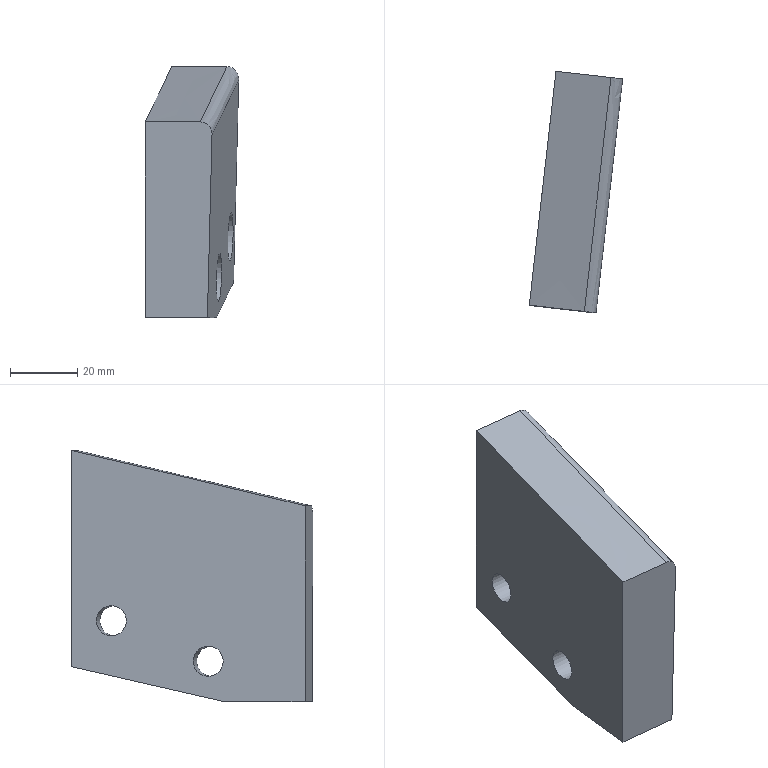Part | NX | features 23 2 | 1 solid | 14 faces | box 27.784 x 71.811 x 74.655 mm | volume 80432 mm3 | plane 8 | cylinder 4 | spline 2 | commonest cylinder face diameters 9 x2 14.5 x2
STEP:
#1=CARTESIAN_POINT('',(2633.571,-359.365,-128.));
#2=VERTEX_POINT('',#1);
#3=CARTESIAN_POINT('',(2638.723,-314.145,-117.631));
#4=VERTEX_POINT('',#3);
#5=CARTESIAN_POINT('',(2657.951,-145.383,-78.935));
#6=DIRECTION('',(0.1104,0.9687,0.2221));
#7=VECTOR('',#6,1000.);
#8=LINE('',#5,#7);
#9=EDGE_CURVE('',#2,#4,#8,.T.);
#10=ORIENTED_EDGE('',*,*,#9,.T.);
#11=CARTESIAN_POINT('',(2640.259,-314.32,-57.071));
#12=VERTEX_POINT('',#11);
#13=CARTESIAN_POINT('',(2623.792,-312.444,-706.206));
#14=DIRECTION('',(-0.02536,0.002889,-0.9997));
#15=VECTOR('',#14,1000.);
#16=LINE('',#13,#15);
#17=EDGE_CURVE('',#12,#4,#16,.T.);
#18=ORIENTED_EDGE('',*,*,#17,.F.);
#19=CARTESIAN_POINT('',(2632.322,-383.869,-73.527));
#20=VERTEX_POINT('',#19);
#21=CARTESIAN_POINT('',(2632.322,-383.869,-73.527));
#22=CARTESIAN_POINT('',(2633.665,-372.094,-70.758));
#23=CARTESIAN_POINT('',(2635.008,-360.336,-67.919));
#24=CARTESIAN_POINT('',(2637.654,-337.147,-62.459));
#25=CARTESIAN_POINT('',(2638.957,-325.733,-59.767));
#26=CARTESIAN_POINT('',(2640.259,-314.32,-57.071));
#27=B_SPLINE_CURVE_WITH_KNOTS('',3,(#21,#22,#23,#24,#25,#26),.UNSPECIFIED.,.F.,.F.,(4,2,4),(0.,0.5077,1.),.UNSPECIFIED.);
#28=EDGE_CURVE('',#20,#12,#27,.T.);
#29=ORIENTED_EDGE('',*,*,#28,.F.);
#30=CARTESIAN_POINT('',(2630.94,-383.711,-128.));
#31=VERTEX_POINT('',#30);
#32=CARTESIAN_POINT('',(2632.693,-383.911,-58.888));
#33=DIRECTION('',(0.02536,-0.002889,0.9997));
#34=VECTOR('',#33,1000.);
#35=LINE('',#32,#34);
#36=EDGE_CURVE('',#31,#20,#35,.T.);
#37=ORIENTED_EDGE('',*,*,#36,.F.);
#38=CARTESIAN_POINT('',(2667.603,-44.391,-128.));
#39=DIRECTION('',(-0.1074,-0.9942,0.));
#40=VECTOR('',#39,1000.);
#41=LINE('',#38,#40);
#42=EDGE_CURVE('',#2,#31,#41,.T.);
#43=ORIENTED_EDGE('',*,*,#42,.F.);
#44=EDGE_LOOP('',(#10,#18,#29,#37,#43));
#45=FACE_BOUND('',#44,.T.);
#46=CARTESIAN_POINT('',(2637.773,-324.494,-111.069));
#47=VERTEX_POINT('',#46);
#48=CARTESIAN_POINT('',(2637.779,-326.115,-104.));
#49=DIRECTION('',(0.9939,-0.1074,-0.02552));
#50=DIRECTION('',(-0.0008715,0.2236,-0.9747));
#51=AXIS2_PLACEMENT_3D('',#48,#49,#50);
#52=ELLIPSE('',#51,7.252,7.25);
#53=EDGE_CURVE('',#47,#47,#52,.T.);
#54=ORIENTED_EDGE('',*,*,#53,.F.);
#55=EDGE_LOOP('',(#54));
#56=FACE_BOUND('',#55,.T.);
#57=CARTESIAN_POINT('',(2634.353,-353.292,-123.069));
#58=VERTEX_POINT('',#57);
#59=CARTESIAN_POINT('',(2634.36,-354.913,-116.));
#60=DIRECTION('',(-0.9939,0.1074,0.02552));
#61=DIRECTION('',(-0.0008715,0.2236,-0.9747));
#62=AXIS2_PLACEMENT_3D('',#59,#60,#61);
#63=ELLIPSE('',#62,7.252,7.25);
#64=EDGE_CURVE('',#58,#58,#63,.T.);
#65=ORIENTED_EDGE('',*,*,#64,.T.);
#66=EDGE_LOOP('',(#65));
#67=FACE_BOUND('',#66,.T.);
#68=CARTESIAN_POINT('',(2489.055,-1559.415,-706.392));
#69=DIRECTION('',(0.9939,-0.1074,-0.02552));
#70=DIRECTION('',(-0.02537,0.002816,-0.9997));
#71=AXIS2_PLACEMENT_3D('',#68,#69,#70);
#72=PLANE('',#71);
#73=ADVANCED_FACE('',(#45,#56,#67),#72,.T.);
#74=CARTESIAN_POINT('',(2612.476,-381.608,-128.));
#75=VERTEX_POINT('',#74);
#76=CARTESIAN_POINT('',(2612.476,-381.608,-69.797));
#77=VERTEX_POINT('',#76);
#78=CARTESIAN_POINT('',(2612.476,-381.608,-57.626));
#79=DIRECTION('',(-0.000000001,0.,1.));
#80=VECTOR('',#79,1000.);
#81=LINE('',#78,#80);
#82=EDGE_CURVE('',#75,#77,#81,.T.);
#83=ORIENTED_EDGE('',*,*,#82,.F.);
#84=CARTESIAN_POINT('',(2583.583,-378.316,-128.));
#85=DIRECTION('',(0.9936,-0.1132,0.));
#86=VECTOR('',#85,1000.);
#87=LINE('',#84,#86);
#88=EDGE_CURVE('',#75,#31,#87,.T.);
#89=ORIENTED_EDGE('',*,*,#88,.T.);
#90=ORIENTED_EDGE('',*,*,#36,.T.);
#91=CARTESIAN_POINT('',(2628.846,-383.473,-69.839));
#92=VERTEX_POINT('',#91);
#93=CARTESIAN_POINT('',(2632.322,-383.869,-73.527));
#94=CARTESIAN_POINT('',(2632.346,-383.872,-72.575));
#95=CARTESIAN_POINT('',(2631.639,-383.791,-70.68));
#96=CARTESIAN_POINT('',(2629.793,-383.581,-69.839));
#97=CARTESIAN_POINT('',(2628.846,-383.473,-69.839));
#98=B_SPLINE_CURVE_WITH_KNOTS('',3,(#93,#94,#95,#96,#97),.UNSPECIFIED.,.F.,.F.,(4,1,4),(0.,0.002818,0.005635),.UNSPECIFIED.);
#99=EDGE_CURVE('',#20,#92,#98,.T.);
#100=ORIENTED_EDGE('',*,*,#99,.T.);
#101=CARTESIAN_POINT('',(2612.476,-381.608,-69.797));
#102=CARTESIAN_POINT('',(2617.932,-382.229,-69.828));
#103=CARTESIAN_POINT('',(2623.389,-382.851,-69.838));
#104=CARTESIAN_POINT('',(2628.846,-383.473,-69.839));
#105=B_SPLINE_CURVE_WITH_KNOTS('',3,(#101,#102,#103,#104),.UNSPECIFIED.,.F.,.F.,(4,4),(0.,0.01648),.UNSPECIFIED.);
#106=EDGE_CURVE('',#77,#92,#105,.T.);
#107=ORIENTED_EDGE('',*,*,#106,.F.);
#108=EDGE_LOOP('',(#83,#89,#90,#100,#107));
#109=FACE_BOUND('',#108,.T.);
#110=CARTESIAN_POINT('',(2583.583,-378.316,-57.626));
#111=DIRECTION('',(-0.1132,-0.9936,0.));
#112=DIRECTION('',(0.02514,-0.002864,0.9997));
#113=AXIS2_PLACEMENT_3D('',#110,#111,#112);
#114=PLANE('',#113);
#115=ADVANCED_FACE('',(#109),#114,.T.);
#116=CARTESIAN_POINT('',(2616.268,-348.323,-116.));
#117=VERTEX_POINT('',#116);
#118=CARTESIAN_POINT('',(2615.759,-352.794,-116.));
#119=DIRECTION('',(0.9936,-0.1132,0.000000001));
#120=DIRECTION('',(0.1132,0.9936,0.));
#121=AXIS2_PLACEMENT_3D('',#118,#119,#120);
#122=CIRCLE('',#121,4.5);
#123=EDGE_CURVE('',#117,#117,#122,.T.);
#124=ORIENTED_EDGE('',*,*,#123,.T.);
#125=EDGE_LOOP('',(#124));
#126=FACE_BOUND('',#125,.T.);
#127=CARTESIAN_POINT('',(2619.551,-319.509,-104.));
#128=VERTEX_POINT('',#127);
#129=CARTESIAN_POINT('',(2619.041,-323.98,-104.));
#130=DIRECTION('',(0.9936,-0.1132,0.000000001));
#131=DIRECTION('',(0.1132,0.9936,0.));
#132=AXIS2_PLACEMENT_3D('',#129,#130,#131);
#133=CIRCLE('',#132,4.5);
#134=EDGE_CURVE('',#128,#128,#133,.T.);
#135=ORIENTED_EDGE('',*,*,#134,.T.);
#136=EDGE_LOOP('',(#135));
#137=FACE_BOUND('',#136,.T.);
#138=CARTESIAN_POINT('',(2620.4,-312.058,-53.345));
#139=VERTEX_POINT('',#138);
#140=CARTESIAN_POINT('',(2620.4,-312.058,-117.631));
#141=VERTEX_POINT('',#140);
#142=CARTESIAN_POINT('',(2620.4,-312.058,-77.534));
#143=DIRECTION('',(0.000000001,0.,-1.));
#144=VECTOR('',#143,1000.);
#145=LINE('',#142,#144);
#146=EDGE_CURVE('',#139,#141,#145,.T.);
#147=ORIENTED_EDGE('',*,*,#146,.T.);
#148=CARTESIAN_POINT('',(2615.248,-357.277,-128.));
#149=VERTEX_POINT('',#148);
#150=CARTESIAN_POINT('',(2624.635,-274.889,-109.109));
#151=DIRECTION('',(-0.1104,-0.9687,-0.2221));
#152=VECTOR('',#151,1000.);
#153=LINE('',#150,#152);
#154=EDGE_CURVE('',#141,#149,#153,.T.);
#155=ORIENTED_EDGE('',*,*,#154,.T.);
#156=CARTESIAN_POINT('',(2649.656,-55.283,-128.));
#157=DIRECTION('',(0.1132,0.9936,0.));
#158=VECTOR('',#157,1000.);
#159=LINE('',#156,#158);
#160=EDGE_CURVE('',#75,#149,#159,.T.);
#161=ORIENTED_EDGE('',*,*,#160,.F.);
#162=ORIENTED_EDGE('',*,*,#82,.T.);
#163=CARTESIAN_POINT('',(2620.4,-312.058,-53.345));
#164=CARTESIAN_POINT('',(2619.079,-323.652,-56.075));
#165=CARTESIAN_POINT('',(2617.429,-338.135,-59.531));
#166=CARTESIAN_POINT('',(2615.445,-355.549,-63.527));
#167=CARTESIAN_POINT('',(2614.455,-364.231,-65.635));
#168=CARTESIAN_POINT('',(2613.468,-372.901,-67.793));
#169=CARTESIAN_POINT('',(2612.806,-378.706,-69.127));
#170=CARTESIAN_POINT('',(2612.476,-381.608,-69.797));
#171=B_SPLINE_CURVE_WITH_KNOTS('',3,(#163,#164,#165,#166,#167,#168,#169,#170),.UNSPECIFIED.,.F.,.F.,(4,1,1,1,1,4),(0.000000001,0.03595,0.04494,0.05393,0.06292,0.07191),.UNSPECIFIED.);
#172=EDGE_CURVE('',#139,#77,#171,.T.);
#173=ORIENTED_EDGE('',*,*,#172,.F.);
#174=EDGE_LOOP('',(#147,#155,#161,#162,#173));
#175=FACE_BOUND('',#174,.T.);
#176=CARTESIAN_POINT('',(2623.82,-282.036,-77.534));
#177=DIRECTION('',(0.9936,-0.1132,0.000000001));
#178=DIRECTION('',(-0.1132,-0.9936,0.));
#179=AXIS2_PLACEMENT_3D('',#176,#177,#178);
#180=PLANE('',#179);
#181=ADVANCED_FACE('',(#126,#137,#175),#180,.F.);
#182=CARTESIAN_POINT('',(2636.764,-313.922,-53.382));
#183=VERTEX_POINT('',#182);
#184=CARTESIAN_POINT('',(2628.846,-383.473,-69.839));
#185=CARTESIAN_POINT('',(2629.501,-377.671,-68.474));
#186=CARTESIAN_POINT('',(2630.852,-366.067,-65.696));
#187=CARTESIAN_POINT('',(2633.434,-342.919,-60.21));
#188=CARTESIAN_POINT('',(2635.437,-325.509,-56.118));
#189=CARTESIAN_POINT('',(2636.764,-313.922,-53.382));
#190=B_SPLINE_CURVE_WITH_KNOTS('',3,(#184,#185,#186,#187,#188,#189),.UNSPECIFIED.,.F.,.F.,(4,1,1,4),(0.,0.25,0.5,1.),.UNSPECIFIED.);
#191=EDGE_CURVE('',#183,#92,#190,.F.);
#192=ORIENTED_EDGE('',*,*,#191,.F.);
#193=CARTESIAN_POINT('',(2620.4,-312.058,-53.345));
#194=CARTESIAN_POINT('',(2625.855,-312.679,-53.392));
#195=CARTESIAN_POINT('',(2631.31,-313.301,-53.411));
#196=CARTESIAN_POINT('',(2636.764,-313.922,-53.382));
#197=B_SPLINE_CURVE_WITH_KNOTS('',3,(#193,#194,#195,#196),.UNSPECIFIED.,.F.,.F.,(4,4),(0.,0.01647),.UNSPECIFIED.);
#198=EDGE_CURVE('',#139,#183,#197,.T.);
#199=ORIENTED_EDGE('',*,*,#198,.F.);
#200=ORIENTED_EDGE('',*,*,#172,.T.);
#201=ORIENTED_EDGE('',*,*,#106,.T.);
#202=EDGE_LOOP('',(#192,#199,#200,#201));
#203=FACE_BOUND('',#202,.T.);
#204=CARTESIAN_POINT('',(2636.914,-313.483,-53.275));
#205=CARTESIAN_POINT('',(2636.252,-319.35,-54.66));
#206=CARTESIAN_POINT('',(2635.591,-325.219,-56.05));
#207=CARTESIAN_POINT('',(2634.277,-336.961,-58.819));
#208=CARTESIAN_POINT('',(2633.616,-342.834,-60.198));
#209=CARTESIAN_POINT('',(2632.794,-350.17,-61.925));
#210=CARTESIAN_POINT('',(2632.631,-351.637,-62.271));
#211=CARTESIAN_POINT('',(2632.302,-354.573,-62.962));
#212=CARTESIAN_POINT('',(2632.139,-356.039,-63.307));
#213=CARTESIAN_POINT('',(2631.661,-360.437,-64.348));
#214=CARTESIAN_POINT('',(2631.339,-363.365,-65.048));
#215=CARTESIAN_POINT('',(2630.676,-369.23,-66.454));
#216=CARTESIAN_POINT('',(2630.342,-372.166,-67.157));
#217=CARTESIAN_POINT('',(2629.68,-378.04,-68.552));
#218=CARTESIAN_POINT('',(2629.352,-380.978,-69.246));
#219=CARTESIAN_POINT('',(2629.026,-383.916,-69.937));
#220=CARTESIAN_POINT('',(2634.148,-313.169,-53.29));
#221=CARTESIAN_POINT('',(2633.484,-319.037,-54.674));
#222=CARTESIAN_POINT('',(2632.816,-324.904,-56.062));
#223=CARTESIAN_POINT('',(2631.504,-336.645,-58.834));
#224=CARTESIAN_POINT('',(2630.844,-342.522,-60.213));
#225=CARTESIAN_POINT('',(2630.023,-349.855,-61.939));
#226=CARTESIAN_POINT('',(2629.86,-351.324,-62.285));
#227=CARTESIAN_POINT('',(2629.531,-354.259,-62.976));
#228=CARTESIAN_POINT('',(2629.368,-355.719,-63.32));
#229=CARTESIAN_POINT('',(2628.888,-360.103,-64.369));
#230=CARTESIAN_POINT('',(2628.562,-363.04,-65.08));
#231=CARTESIAN_POINT('',(2627.896,-368.912,-66.487));
#232=CARTESIAN_POINT('',(2627.558,-371.854,-67.186));
#233=CARTESIAN_POINT('',(2626.89,-377.733,-68.567));
#234=CARTESIAN_POINT('',(2626.558,-380.672,-69.252));
#235=CARTESIAN_POINT('',(2626.23,-383.607,-69.938));
#236=CARTESIAN_POINT('',(2631.371,-312.854,-53.311));
#237=CARTESIAN_POINT('',(2630.709,-318.725,-54.693));
#238=CARTESIAN_POINT('',(2630.042,-324.591,-56.072));
#239=CARTESIAN_POINT('',(2628.722,-336.328,-58.844));
#240=CARTESIAN_POINT('',(2628.066,-342.21,-60.226));
#241=CARTESIAN_POINT('',(2627.246,-349.541,-61.95));
#242=CARTESIAN_POINT('',(2627.081,-351.01,-62.297));
#243=CARTESIAN_POINT('',(2626.75,-353.947,-62.987));
#244=CARTESIAN_POINT('',(2626.585,-355.405,-63.329));
#245=CARTESIAN_POINT('',(2626.085,-359.783,-64.378));
#246=CARTESIAN_POINT('',(2625.754,-362.721,-65.091));
#247=CARTESIAN_POINT('',(2625.101,-368.596,-66.497));
#248=CARTESIAN_POINT('',(2624.773,-371.54,-67.195));
#249=CARTESIAN_POINT('',(2624.107,-377.422,-68.573));
#250=CARTESIAN_POINT('',(2623.772,-380.361,-69.256));
#251=CARTESIAN_POINT('',(2623.44,-383.299,-69.939));
#252=CARTESIAN_POINT('',(2625.797,-312.231,-53.295));
#253=CARTESIAN_POINT('',(2625.138,-318.105,-54.675));
#254=CARTESIAN_POINT('',(2624.479,-323.974,-56.05));
#255=CARTESIAN_POINT('',(2623.153,-335.712,-58.815));
#256=CARTESIAN_POINT('',(2622.491,-341.592,-60.192));
#257=CARTESIAN_POINT('',(2621.675,-348.915,-61.925));
#258=CARTESIAN_POINT('',(2621.511,-350.389,-62.276));
#259=CARTESIAN_POINT('',(2621.176,-353.342,-62.963));
#260=CARTESIAN_POINT('',(2621.006,-354.806,-63.299));
#261=CARTESIAN_POINT('',(2620.499,-359.187,-64.324));
#262=CARTESIAN_POINT('',(2620.175,-362.102,-65.031));
#263=CARTESIAN_POINT('',(2619.534,-367.963,-66.459));
#264=CARTESIAN_POINT('',(2619.21,-370.909,-67.173));
#265=CARTESIAN_POINT('',(2618.541,-376.797,-68.565));
#266=CARTESIAN_POINT('',(2618.201,-379.74,-69.249));
#267=CARTESIAN_POINT('',(2617.862,-382.681,-69.929));
#268=CARTESIAN_POINT('',(2623.027,-311.926,-53.267));
#269=CARTESIAN_POINT('',(2622.368,-317.799,-54.649));
#270=CARTESIAN_POINT('',(2621.711,-323.668,-56.024));
#271=CARTESIAN_POINT('',(2620.393,-335.409,-58.788));
#272=CARTESIAN_POINT('',(2619.72,-341.296,-60.158));
#273=CARTESIAN_POINT('',(2618.913,-348.607,-61.894));
#274=CARTESIAN_POINT('',(2618.753,-350.085,-62.249));
#275=CARTESIAN_POINT('',(2618.408,-353.053,-62.934));
#276=CARTESIAN_POINT('',(2618.23,-354.52,-63.263));
#277=CARTESIAN_POINT('',(2617.72,-358.899,-64.27));
#278=CARTESIAN_POINT('',(2617.407,-361.796,-64.976));
#279=CARTESIAN_POINT('',(2616.775,-367.646,-66.424));
#280=CARTESIAN_POINT('',(2616.448,-370.596,-67.152));
#281=CARTESIAN_POINT('',(2615.764,-376.487,-68.555));
#282=CARTESIAN_POINT('',(2615.413,-379.43,-69.239));
#283=CARTESIAN_POINT('',(2615.072,-382.372,-69.919));
#284=CARTESIAN_POINT('',(2620.261,-311.619,-53.246));
#285=CARTESIAN_POINT('',(2619.601,-317.492,-54.628));
#286=CARTESIAN_POINT('',(2618.944,-323.361,-56.005));
#287=CARTESIAN_POINT('',(2617.626,-335.103,-58.769));
#288=CARTESIAN_POINT('',(2616.959,-340.995,-60.134));
#289=CARTESIAN_POINT('',(2616.143,-348.296,-61.873));
#290=CARTESIAN_POINT('',(2615.979,-349.776,-62.23));
#291=CARTESIAN_POINT('',(2615.643,-352.751,-62.915));
#292=CARTESIAN_POINT('',(2615.476,-354.216,-63.241));
#293=CARTESIAN_POINT('',(2614.992,-358.589,-64.25));
#294=CARTESIAN_POINT('',(2614.675,-361.488,-64.964));
#295=CARTESIAN_POINT('',(2614.016,-367.336,-66.419));
#296=CARTESIAN_POINT('',(2613.674,-370.288,-67.148));
#297=CARTESIAN_POINT('',(2612.98,-376.181,-68.546));
#298=CARTESIAN_POINT('',(2612.629,-379.125,-69.226));
#299=CARTESIAN_POINT('',(2612.285,-382.063,-69.905));
#300=B_SPLINE_SURFACE_WITH_KNOTS('',3,3,((#204,#205,#206,#207,#208,#209,#210,#211,#212,#213,#214,#215,#216,#217,#218,#219),(#220,#221,#222,#223,#224,#225,#226,#227,#228,#229,#230,#231,#232,#233,#234,#235),(#236,#237,#238,#239,#240,#241,#242,#243,#244,#245,#246,#247,#248,#249,#250,#251),(#252,#253,#254,#255,#256,#257,#258,#259,#260,#261,#262,#263,#264,#265,#266,#267),(#268,#269,#270,#271,#272,#273,#274,#275,#276,#277,#278,#279,#280,#281,#282,#283),(#284,#285,#286,#287,#288,#289,#290,#291,#292,#293,#294,#295,#296,#297,#298,#299)),.UNSPECIFIED.,.F.,.F.,.F.,(4,2,4),(4,2,2,2,2,2,2,4),(0.,0.5,1.),(0.,0.25,0.5,0.5625,0.625,0.75,0.875,1.),.UNSPECIFIED.);
#301=ADVANCED_FACE('',(#203),#300,.T.);
#302=CARTESIAN_POINT('',(436.092,-108.994,-128.));
#303=DIRECTION('',(-0.9936,0.1132,0.));
#304=VECTOR('',#303,1000.);
#305=LINE('',#302,#304);
#306=EDGE_CURVE('',#2,#149,#305,.T.);
#307=ORIENTED_EDGE('',*,*,#306,.F.);
#308=ORIENTED_EDGE('',*,*,#42,.T.);
#309=ORIENTED_EDGE('',*,*,#88,.F.);
#310=ORIENTED_EDGE('',*,*,#160,.T.);
#311=EDGE_LOOP('',(#307,#308,#309,#310));
#312=FACE_BOUND('',#311,.T.);
#313=CARTESIAN_POINT('',(470.5,193.,-128.));
#314=DIRECTION('',(0.,0.,-1.));
#315=DIRECTION('',(-1.,0.,0.));
#316=AXIS2_PLACEMENT_3D('',#313,#314,#315);
#317=PLANE('',#316);
#318=ADVANCED_FACE('',(#312),#317,.T.);
#319=CARTESIAN_POINT('',(2640.259,-314.32,-57.071));
#320=CARTESIAN_POINT('',(2640.283,-314.323,-56.115));
#321=CARTESIAN_POINT('',(2639.571,-314.242,-54.214));
#322=CARTESIAN_POINT('',(2637.715,-314.03,-53.376));
#323=CARTESIAN_POINT('',(2636.764,-313.922,-53.382));
#324=B_SPLINE_CURVE_WITH_KNOTS('',3,(#319,#320,#321,#322,#323),.UNSPECIFIED.,.F.,.F.,(4,1,4),(0.,0.002827,0.005654),.UNSPECIFIED.);
#325=EDGE_CURVE('',#12,#183,#324,.T.);
#326=ORIENTED_EDGE('',*,*,#325,.T.);
#327=ORIENTED_EDGE('',*,*,#191,.T.);
#328=ORIENTED_EDGE('',*,*,#99,.F.);
#329=ORIENTED_EDGE('',*,*,#28,.T.);
#330=EDGE_LOOP('',(#326,#327,#328,#329));
#331=FACE_BOUND('',#330,.T.);
#332=CARTESIAN_POINT('',(2636.783,-313.496,-53.282));
#333=CARTESIAN_POINT('',(2637.204,-313.545,-53.28));
#334=CARTESIAN_POINT('',(2637.66,-313.581,-53.347));
#335=CARTESIAN_POINT('',(2638.554,-313.602,-53.687));
#336=CARTESIAN_POINT('',(2638.986,-313.588,-53.958));
#337=CARTESIAN_POINT('',(2639.7,-313.505,-54.654));
#338=CARTESIAN_POINT('',(2639.978,-313.437,-55.076));
#339=CARTESIAN_POINT('',(2640.33,-313.271,-55.95));
#340=CARTESIAN_POINT('',(2640.4,-313.173,-56.397));
#341=CARTESIAN_POINT('',(2640.4,-313.076,-56.809));
#342=CARTESIAN_POINT('',(2635.432,-325.371,-56.085));
#343=CARTESIAN_POINT('',(2635.853,-325.419,-56.084));
#344=CARTESIAN_POINT('',(2636.309,-325.455,-56.152));
#345=CARTESIAN_POINT('',(2637.202,-325.476,-56.492));
#346=CARTESIAN_POINT('',(2637.634,-325.461,-56.763));
#347=CARTESIAN_POINT('',(2638.346,-325.377,-57.458));
#348=CARTESIAN_POINT('',(2638.624,-325.309,-57.88));
#349=CARTESIAN_POINT('',(2638.975,-325.141,-58.753));
#350=CARTESIAN_POINT('',(2639.046,-325.043,-59.199));
#351=CARTESIAN_POINT('',(2639.046,-324.945,-59.612));
#352=CARTESIAN_POINT('',(2634.077,-337.229,-58.884));
#353=CARTESIAN_POINT('',(2634.498,-337.277,-58.882));
#354=CARTESIAN_POINT('',(2634.954,-337.314,-58.949));
#355=CARTESIAN_POINT('',(2635.847,-337.336,-59.29));
#356=CARTESIAN_POINT('',(2636.279,-337.322,-59.561));
#357=CARTESIAN_POINT('',(2636.992,-337.24,-60.257));
#358=CARTESIAN_POINT('',(2637.27,-337.173,-60.679));
#359=CARTESIAN_POINT('',(2637.621,-337.008,-61.553));
#360=CARTESIAN_POINT('',(2637.691,-336.912,-62.));
#361=CARTESIAN_POINT('',(2637.691,-336.815,-62.413));
#362=CARTESIAN_POINT('',(2632.044,-355.042,-63.078));
#363=CARTESIAN_POINT('',(2632.465,-355.09,-63.076));
#364=CARTESIAN_POINT('',(2632.922,-355.126,-63.144));
#365=CARTESIAN_POINT('',(2633.815,-355.148,-63.484));
#366=CARTESIAN_POINT('',(2634.247,-355.133,-63.755));
#367=CARTESIAN_POINT('',(2634.96,-355.05,-64.451));
#368=CARTESIAN_POINT('',(2635.238,-354.982,-64.873));
#369=CARTESIAN_POINT('',(2635.589,-354.816,-65.747));
#370=CARTESIAN_POINT('',(2635.66,-354.719,-66.193));
#371=CARTESIAN_POINT('',(2635.66,-354.621,-66.606));
#372=CARTESIAN_POINT('',(2631.34,-360.985,-64.488));
#373=CARTESIAN_POINT('',(2631.762,-361.034,-64.483));
#374=CARTESIAN_POINT('',(2632.221,-361.071,-64.547));
#375=CARTESIAN_POINT('',(2633.12,-361.093,-64.884));
#376=CARTESIAN_POINT('',(2633.556,-361.078,-65.154));
#377=CARTESIAN_POINT('',(2634.276,-360.993,-65.85));
#378=CARTESIAN_POINT('',(2634.557,-360.923,-66.274));
#379=CARTESIAN_POINT('',(2634.911,-360.753,-67.15));
#380=CARTESIAN_POINT('',(2634.982,-360.654,-67.598));
#381=CARTESIAN_POINT('',(2634.983,-360.555,-68.012));
#382=CARTESIAN_POINT('',(2629.991,-372.843,-67.33));
#383=CARTESIAN_POINT('',(2630.413,-372.892,-67.326));
#384=CARTESIAN_POINT('',(2630.871,-372.929,-67.391));
#385=CARTESIAN_POINT('',(2631.769,-372.951,-67.729));
#386=CARTESIAN_POINT('',(2632.205,-372.936,-67.999));
#387=CARTESIAN_POINT('',(2632.923,-372.851,-68.695));
#388=CARTESIAN_POINT('',(2633.203,-372.782,-69.118));
#389=CARTESIAN_POINT('',(2633.557,-372.612,-69.994));
#390=CARTESIAN_POINT('',(2633.628,-372.513,-70.442));
#391=CARTESIAN_POINT('',(2633.628,-372.414,-70.855));
#392=CARTESIAN_POINT('',(2629.346,-378.766,-68.733));
#393=CARTESIAN_POINT('',(2629.767,-378.814,-68.732));
#394=CARTESIAN_POINT('',(2630.222,-378.85,-68.801));
#395=CARTESIAN_POINT('',(2631.113,-378.871,-69.143));
#396=CARTESIAN_POINT('',(2631.543,-378.857,-69.414));
#397=CARTESIAN_POINT('',(2632.254,-378.774,-70.11));
#398=CARTESIAN_POINT('',(2632.531,-378.707,-70.531));
#399=CARTESIAN_POINT('',(2632.881,-378.542,-71.404));
#400=CARTESIAN_POINT('',(2632.951,-378.445,-71.849));
#401=CARTESIAN_POINT('',(2632.951,-378.348,-72.262));
#402=CARTESIAN_POINT('',(2628.677,-384.703,-70.129));
#403=CARTESIAN_POINT('',(2629.097,-384.751,-70.129));
#404=CARTESIAN_POINT('',(2629.552,-384.786,-70.199));
#405=CARTESIAN_POINT('',(2630.441,-384.807,-70.541));
#406=CARTESIAN_POINT('',(2630.87,-384.793,-70.813));
#407=CARTESIAN_POINT('',(2631.579,-384.71,-71.508));
#408=CARTESIAN_POINT('',(2631.855,-384.642,-71.929));
#409=CARTESIAN_POINT('',(2632.204,-384.477,-72.8));
#410=CARTESIAN_POINT('',(2632.274,-384.381,-73.245));
#411=CARTESIAN_POINT('',(2632.274,-384.284,-73.657));
#412=B_SPLINE_SURFACE_WITH_KNOTS('',3,3,((#332,#333,#334,#335,#336,#337,#338,#339,#340,#341),(#342,#343,#344,#345,#346,#347,#348,#349,#350,#351),(#352,#353,#354,#355,#356,#357,#358,#359,#360,#361),(#362,#363,#364,#365,#366,#367,#368,#369,#370,#371),(#372,#373,#374,#375,#376,#377,#378,#379,#380,#381),(#382,#383,#384,#385,#386,#387,#388,#389,#390,#391),(#392,#393,#394,#395,#396,#397,#398,#399,#400,#401),(#402,#403,#404,#405,#406,#407,#408,#409,#410,#411)),.UNSPECIFIED.,.F.,.F.,.F.,(4,2,2,4),(4,2,2,2,4),(0.,0.5,0.75,1.),(-0.006005,0.2471,0.5002,0.7532,1.006),.UNSPECIFIED.);
#413=ADVANCED_FACE('',(#331),#412,.T.);
#414=ORIENTED_EDGE('',*,*,#17,.T.);
#415=CARTESIAN_POINT('',(2630.336,-313.19,-117.631));
#416=DIRECTION('',(-0.9936,0.1132,-0.000000001));
#417=VECTOR('',#416,1000.);
#418=LINE('',#415,#417);
#419=EDGE_CURVE('',#4,#141,#418,.T.);
#420=ORIENTED_EDGE('',*,*,#419,.T.);
#421=ORIENTED_EDGE('',*,*,#146,.F.);
#422=ORIENTED_EDGE('',*,*,#198,.T.);
#423=ORIENTED_EDGE('',*,*,#325,.F.);
#424=EDGE_LOOP('',(#414,#420,#421,#422,#423));
#425=FACE_BOUND('',#424,.T.);
#426=CARTESIAN_POINT('',(2630.336,-313.19,-98.495));
#427=DIRECTION('',(-0.1132,-0.9936,0.));
#428=DIRECTION('',(-0.9936,0.1132,0.));
#429=AXIS2_PLACEMENT_3D('',#426,#427,#428);
#430=PLANE('',#429);
#431=ADVANCED_FACE('',(#425),#430,.F.);
#432=CARTESIAN_POINT('',(2628.493,-320.528,-104.));
#433=VERTEX_POINT('',#432);
#434=CARTESIAN_POINT('',(2627.984,-324.999,-104.));
#435=DIRECTION('',(0.9936,-0.1132,0.000000001));
#436=DIRECTION('',(0.1132,0.9936,0.));
#437=AXIS2_PLACEMENT_3D('',#434,#435,#436);
#438=CIRCLE('',#437,4.5);
#439=EDGE_CURVE('',#433,#433,#438,.T.);
#440=ORIENTED_EDGE('',*,*,#439,.T.);
#441=EDGE_LOOP('',(#440));
#442=FACE_BOUND('',#441,.T.);
#443=ORIENTED_EDGE('',*,*,#134,.F.);
#444=EDGE_LOOP('',(#443));
#445=FACE_BOUND('',#444,.T.);
#446=CARTESIAN_POINT('',(2638.913,-326.245,-104.));
#447=DIRECTION('',(-0.9936,0.1132,-0.000000001));
#448=DIRECTION('',(0.01281,0.1125,-0.9936));
#449=AXIS2_PLACEMENT_3D('',#446,#447,#448);
#450=CYLINDRICAL_SURFACE('',#449,4.5);
#451=ADVANCED_FACE('',(#442,#445),#450,.F.);
#452=ORIENTED_EDGE('',*,*,#439,.F.);
#453=EDGE_LOOP('',(#452));
#454=FACE_BOUND('',#453,.T.);
#455=CARTESIAN_POINT('',(2627.891,-325.815,-96.797));
#456=VERTEX_POINT('',#455);
#457=CARTESIAN_POINT('',(2627.984,-324.999,-104.));
#458=DIRECTION('',(0.9936,-0.1132,0.000000001));
#459=DIRECTION('',(-0.01281,-0.1125,0.9936));
#460=AXIS2_PLACEMENT_3D('',#457,#458,#459);
#461=CIRCLE('',#460,7.25);
#462=EDGE_CURVE('',#456,#456,#461,.T.);
#463=ORIENTED_EDGE('',*,*,#462,.T.);
#464=EDGE_LOOP('',(#463));
#465=FACE_BOUND('',#464,.T.);
#466=CARTESIAN_POINT('',(2627.984,-324.999,-87.));
#467=DIRECTION('',(-0.9936,0.1132,-0.000000001));
#468=DIRECTION('',(-0.1132,-0.9936,0.));
#469=AXIS2_PLACEMENT_3D('',#466,#467,#468);
#470=PLANE('',#469);
#471=ADVANCED_FACE('',(#454,#465),#470,.F.);
#472=ORIENTED_EDGE('',*,*,#462,.F.);
#473=EDGE_LOOP('',(#472));
#474=FACE_BOUND('',#473,.T.);
#475=ORIENTED_EDGE('',*,*,#53,.T.);
#476=EDGE_LOOP('',(#475));
#477=FACE_BOUND('',#476,.T.);
#478=CARTESIAN_POINT('',(2638.913,-326.245,-104.));
#479=DIRECTION('',(-0.9936,0.1132,-0.000000001));
#480=DIRECTION('',(0.01281,0.1125,-0.9936));
#481=AXIS2_PLACEMENT_3D('',#478,#479,#480);
#482=CYLINDRICAL_SURFACE('',#481,7.25);
#483=ADVANCED_FACE('',(#474,#477),#482,.F.);
#484=CARTESIAN_POINT('',(2624.191,-358.284,-116.));
#485=VERTEX_POINT('',#484);
#486=CARTESIAN_POINT('',(2624.701,-353.813,-116.));
#487=DIRECTION('',(-0.9936,0.1132,-0.000000001));
#488=DIRECTION('',(-0.1132,-0.9936,0.));
#489=AXIS2_PLACEMENT_3D('',#486,#487,#488);
#490=CIRCLE('',#489,4.5);
#491=EDGE_CURVE('',#485,#485,#490,.T.);
#492=ORIENTED_EDGE('',*,*,#491,.F.);
#493=EDGE_LOOP('',(#492));
#494=FACE_BOUND('',#493,.T.);
#495=ORIENTED_EDGE('',*,*,#123,.F.);
#496=EDGE_LOOP('',(#495));
#497=FACE_BOUND('',#496,.T.);
#498=CARTESIAN_POINT('',(2635.63,-355.058,-116.));
#499=DIRECTION('',(-0.9936,0.1132,-0.000000001));
#500=DIRECTION('',(-0.01281,-0.1125,-0.9936));
#501=AXIS2_PLACEMENT_3D('',#498,#499,#500);
#502=CYLINDRICAL_SURFACE('',#501,4.5);
#503=ADVANCED_FACE('',(#494,#497),#502,.F.);
#504=ORIENTED_EDGE('',*,*,#491,.T.);
#505=EDGE_LOOP('',(#504));
#506=FACE_BOUND('',#505,.T.);
#507=CARTESIAN_POINT('',(2624.794,-352.997,-108.797));
#508=VERTEX_POINT('',#507);
#509=CARTESIAN_POINT('',(2624.701,-353.813,-116.));
#510=DIRECTION('',(-0.9936,0.1132,-0.000000001));
#511=DIRECTION('',(0.01281,0.1125,0.9936));
#512=AXIS2_PLACEMENT_3D('',#509,#510,#511);
#513=CIRCLE('',#512,7.25);
#514=EDGE_CURVE('',#508,#508,#513,.T.);
#515=ORIENTED_EDGE('',*,*,#514,.F.);
#516=EDGE_LOOP('',(#515));
#517=FACE_BOUND('',#516,.T.);
#518=CARTESIAN_POINT('',(2624.701,-353.813,-116.));
#519=DIRECTION('',(-0.9936,0.1132,-0.000000001));
#520=DIRECTION('',(0.1132,0.9936,0.));
#521=AXIS2_PLACEMENT_3D('',#518,#519,#520);
#522=PLANE('',#521);
#523=ADVANCED_FACE('',(#506,#517),#522,.F.);
#524=ORIENTED_EDGE('',*,*,#514,.T.);
#525=EDGE_LOOP('',(#524));
#526=FACE_BOUND('',#525,.T.);
#527=ORIENTED_EDGE('',*,*,#64,.F.);
#528=EDGE_LOOP('',(#527));
#529=FACE_BOUND('',#528,.T.);
#530=CARTESIAN_POINT('',(2635.63,-355.058,-116.));
#531=DIRECTION('',(-0.9936,0.1132,-0.000000001));
#532=DIRECTION('',(-0.01281,-0.1125,-0.9936));
#533=AXIS2_PLACEMENT_3D('',#530,#531,#532);
#534=CYLINDRICAL_SURFACE('',#533,7.25);
#535=ADVANCED_FACE('',(#526,#529),#534,.F.);
#536=ORIENTED_EDGE('',*,*,#306,.T.);
#537=ORIENTED_EDGE('',*,*,#154,.F.);
#538=ORIENTED_EDGE('',*,*,#419,.F.);
#539=ORIENTED_EDGE('',*,*,#9,.F.);
#540=EDGE_LOOP('',(#536,#537,#538,#539));
#541=FACE_BOUND('',#540,.T.);
#542=CARTESIAN_POINT('',(-2624.08,456.429,-78.935));
#543=DIRECTION('',(-0.02515,-0.2207,0.975));
#544=DIRECTION('',(0.,0.9753,0.2208));
#545=AXIS2_PLACEMENT_3D('',#542,#543,#544);
#546=PLANE('',#545);
#547=ADVANCED_FACE('',(#541),#546,.F.);
#548=CLOSED_SHELL('',(#73,#115,#181,#301,#318,#413,#431,#451,#471,#483,#503,#523,#535,#547));
#549=MANIFOLD_SOLID_BREP('',#548);
#550=(LENGTH_UNIT()NAMED_UNIT(*)SI_UNIT(.MILLI.,.METRE.));
#551=UNCERTAINTY_MEASURE_WITH_UNIT(LENGTH_MEASURE(0.0893),#550,'','');
#552=(NAMED_UNIT(*)PLANE_ANGLE_UNIT()SI_UNIT($,.RADIAN.));
#553=(NAMED_UNIT(*)SI_UNIT($,.STERADIAN.)SOLID_ANGLE_UNIT());
#554=(GEOMETRIC_REPRESENTATION_CONTEXT(3)GLOBAL_UNCERTAINTY_ASSIGNED_CONTEXT((#551))GLOBAL_UNIT_ASSIGNED_CONTEXT((#550,#552,#553))REPRESENTATION_CONTEXT('',''));
#555=ADVANCED_BREP_SHAPE_REPRESENTATION('',(#549),#554);